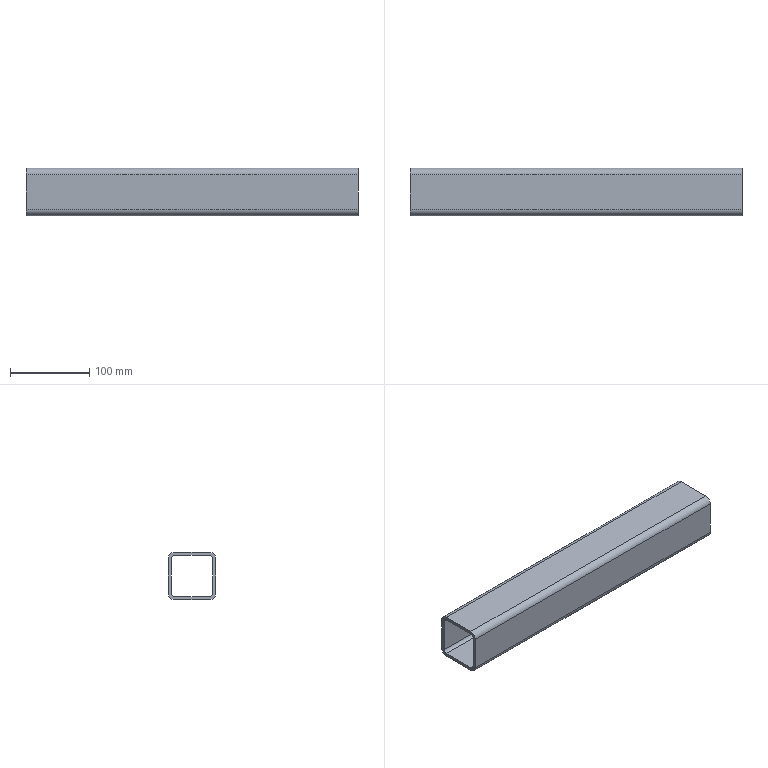Part | SolidWorks | features BaseBody 1 | 1 solid | 18 faces | box 420 x 60 x 60 mm | volume 359015 mm3 | plane 10 | cylinder 8 | commonest cylinder face diameters 8 x4 16 x4
STEP:
#1=CARTESIAN_POINT('',(-210.,2006.,-1308.));
#2=VERTEX_POINT('',#1);
#3=CARTESIAN_POINT('',(210.,2006.,-1308.));
#4=VERTEX_POINT('',#3);
#5=CARTESIAN_POINT('',(-240.,2006.,-1308.));
#6=DIRECTION('',(1.,0.,0.));
#7=VECTOR('',#6,1000.);
#8=LINE('',#5,#7);
#9=EDGE_CURVE('',#2,#4,#8,.T.);
#10=ORIENTED_EDGE('',*,*,#9,.T.);
#11=CARTESIAN_POINT('',(210.,2006.,-1352.));
#12=VERTEX_POINT('',#11);
#13=CARTESIAN_POINT('',(210.,2006.,-1308.));
#14=DIRECTION('',(0.,0.,-1.));
#15=VECTOR('',#14,1000.);
#16=LINE('',#13,#15);
#17=EDGE_CURVE('',#4,#12,#16,.T.);
#18=ORIENTED_EDGE('',*,*,#17,.T.);
#19=CARTESIAN_POINT('',(-210.,2006.,-1352.));
#20=VERTEX_POINT('',#19);
#21=CARTESIAN_POINT('',(-240.,2006.,-1352.));
#22=DIRECTION('',(-1.,0.,0.));
#23=VECTOR('',#22,1000.);
#24=LINE('',#21,#23);
#25=EDGE_CURVE('',#12,#20,#24,.T.);
#26=ORIENTED_EDGE('',*,*,#25,.T.);
#27=CARTESIAN_POINT('',(-210.,2006.,-1308.));
#28=DIRECTION('',(0.,0.,1.));
#29=VECTOR('',#28,1000.);
#30=LINE('',#27,#29);
#31=EDGE_CURVE('',#20,#2,#30,.T.);
#32=ORIENTED_EDGE('',*,*,#31,.T.);
#33=EDGE_LOOP('',(#10,#18,#26,#32));
#34=FACE_OUTER_BOUND('',#33,.T.);
#35=CARTESIAN_POINT('',(-240.,2006.,-1308.));
#36=DIRECTION('',(0.,1.,0.));
#37=DIRECTION('',(0.,0.,1.));
#38=AXIS2_PLACEMENT_3D('',#35,#36,#37);
#39=PLANE('',#38);
#40=ADVANCED_FACE('',(#34),#39,.T.);
#41=CARTESIAN_POINT('',(210.,2010.,-1304.));
#42=VERTEX_POINT('',#41);
#43=CARTESIAN_POINT('',(210.,2010.,-1308.));
#44=DIRECTION('',(1.,0.,0.));
#45=DIRECTION('',(0.,0.,-1.));
#46=AXIS2_PLACEMENT_3D('',#43,#44,#45);
#47=CIRCLE('',#46,4.);
#48=EDGE_CURVE('',#42,#4,#47,.T.);
#49=ORIENTED_EDGE('',*,*,#48,.F.);
#50=CARTESIAN_POINT('',(210.,2054.,-1304.));
#51=VERTEX_POINT('',#50);
#52=CARTESIAN_POINT('',(210.,2054.,-1304.));
#53=DIRECTION('',(0.,-1.,0.));
#54=VECTOR('',#53,1000.);
#55=LINE('',#52,#54);
#56=EDGE_CURVE('',#51,#42,#55,.T.);
#57=ORIENTED_EDGE('',*,*,#56,.F.);
#58=CARTESIAN_POINT('',(210.,2058.,-1308.));
#59=VERTEX_POINT('',#58);
#60=CARTESIAN_POINT('',(210.,2054.,-1308.));
#61=DIRECTION('',(1.,0.,0.));
#62=DIRECTION('',(0.,0.,-1.));
#63=AXIS2_PLACEMENT_3D('',#60,#61,#62);
#64=CIRCLE('',#63,4.);
#65=EDGE_CURVE('',#59,#51,#64,.T.);
#66=ORIENTED_EDGE('',*,*,#65,.F.);
#67=CARTESIAN_POINT('',(210.,2058.,-1352.));
#68=VERTEX_POINT('',#67);
#69=CARTESIAN_POINT('',(210.,2058.,-1352.));
#70=DIRECTION('',(0.,0.,1.));
#71=VECTOR('',#70,1000.);
#72=LINE('',#69,#71);
#73=EDGE_CURVE('',#68,#59,#72,.T.);
#74=ORIENTED_EDGE('',*,*,#73,.F.);
#75=CARTESIAN_POINT('',(210.,2054.,-1356.));
#76=VERTEX_POINT('',#75);
#77=CARTESIAN_POINT('',(210.,2054.,-1352.));
#78=DIRECTION('',(1.,0.,0.));
#79=DIRECTION('',(0.,0.,-1.));
#80=AXIS2_PLACEMENT_3D('',#77,#78,#79);
#81=CIRCLE('',#80,4.);
#82=EDGE_CURVE('',#76,#68,#81,.T.);
#83=ORIENTED_EDGE('',*,*,#82,.F.);
#84=CARTESIAN_POINT('',(210.,2010.,-1356.));
#85=VERTEX_POINT('',#84);
#86=CARTESIAN_POINT('',(210.,2054.,-1356.));
#87=DIRECTION('',(0.,1.,0.));
#88=VECTOR('',#87,1000.);
#89=LINE('',#86,#88);
#90=EDGE_CURVE('',#85,#76,#89,.T.);
#91=ORIENTED_EDGE('',*,*,#90,.F.);
#92=CARTESIAN_POINT('',(210.,2010.,-1352.));
#93=DIRECTION('',(1.,0.,0.));
#94=DIRECTION('',(0.,0.,-1.));
#95=AXIS2_PLACEMENT_3D('',#92,#93,#94);
#96=CIRCLE('',#95,4.);
#97=EDGE_CURVE('',#12,#85,#96,.T.);
#98=ORIENTED_EDGE('',*,*,#97,.F.);
#99=ORIENTED_EDGE('',*,*,#17,.F.);
#100=EDGE_LOOP('',(#49,#57,#66,#74,#83,#91,#98,#99));
#101=FACE_BOUND('',#100,.T.);
#102=CARTESIAN_POINT('',(210.,2054.,-1300.));
#103=VERTEX_POINT('',#102);
#104=CARTESIAN_POINT('',(210.,2062.,-1308.));
#105=VERTEX_POINT('',#104);
#106=CARTESIAN_POINT('',(210.,2054.,-1308.));
#107=DIRECTION('',(-1.,0.,0.));
#108=DIRECTION('',(0.,0.,-1.));
#109=AXIS2_PLACEMENT_3D('',#106,#107,#108);
#110=CIRCLE('',#109,8.);
#111=EDGE_CURVE('',#103,#105,#110,.T.);
#112=ORIENTED_EDGE('',*,*,#111,.F.);
#113=CARTESIAN_POINT('',(210.,2010.,-1300.));
#114=VERTEX_POINT('',#113);
#115=CARTESIAN_POINT('',(210.,2054.,-1300.));
#116=DIRECTION('',(0.,1.,0.));
#117=VECTOR('',#116,1000.);
#118=LINE('',#115,#117);
#119=EDGE_CURVE('',#114,#103,#118,.T.);
#120=ORIENTED_EDGE('',*,*,#119,.F.);
#121=CARTESIAN_POINT('',(210.,2002.,-1308.));
#122=VERTEX_POINT('',#121);
#123=CARTESIAN_POINT('',(210.,2010.,-1308.));
#124=DIRECTION('',(-1.,0.,0.));
#125=DIRECTION('',(0.,0.,-1.));
#126=AXIS2_PLACEMENT_3D('',#123,#124,#125);
#127=CIRCLE('',#126,8.);
#128=EDGE_CURVE('',#122,#114,#127,.T.);
#129=ORIENTED_EDGE('',*,*,#128,.F.);
#130=CARTESIAN_POINT('',(210.,2002.,-1352.));
#131=VERTEX_POINT('',#130);
#132=CARTESIAN_POINT('',(210.,2002.,-1352.));
#133=DIRECTION('',(0.,0.,1.));
#134=VECTOR('',#133,1000.);
#135=LINE('',#132,#134);
#136=EDGE_CURVE('',#131,#122,#135,.T.);
#137=ORIENTED_EDGE('',*,*,#136,.F.);
#138=CARTESIAN_POINT('',(210.,2010.,-1360.));
#139=VERTEX_POINT('',#138);
#140=CARTESIAN_POINT('',(210.,2010.,-1352.));
#141=DIRECTION('',(-1.,0.,0.));
#142=DIRECTION('',(0.,0.,-1.));
#143=AXIS2_PLACEMENT_3D('',#140,#141,#142);
#144=CIRCLE('',#143,8.);
#145=EDGE_CURVE('',#139,#131,#144,.T.);
#146=ORIENTED_EDGE('',*,*,#145,.F.);
#147=CARTESIAN_POINT('',(210.,2054.,-1360.));
#148=VERTEX_POINT('',#147);
#149=CARTESIAN_POINT('',(210.,2054.,-1360.));
#150=DIRECTION('',(0.,-1.,0.));
#151=VECTOR('',#150,1000.);
#152=LINE('',#149,#151);
#153=EDGE_CURVE('',#148,#139,#152,.T.);
#154=ORIENTED_EDGE('',*,*,#153,.F.);
#155=CARTESIAN_POINT('',(210.,2062.,-1352.));
#156=VERTEX_POINT('',#155);
#157=CARTESIAN_POINT('',(210.,2054.,-1352.));
#158=DIRECTION('',(-1.,0.,0.));
#159=DIRECTION('',(0.,0.,-1.));
#160=AXIS2_PLACEMENT_3D('',#157,#158,#159);
#161=CIRCLE('',#160,8.);
#162=EDGE_CURVE('',#156,#148,#161,.T.);
#163=ORIENTED_EDGE('',*,*,#162,.F.);
#164=CARTESIAN_POINT('',(210.,2062.,-1352.));
#165=DIRECTION('',(0.,0.,-1.));
#166=VECTOR('',#165,1000.);
#167=LINE('',#164,#166);
#168=EDGE_CURVE('',#105,#156,#167,.T.);
#169=ORIENTED_EDGE('',*,*,#168,.F.);
#170=EDGE_LOOP('',(#112,#120,#129,#137,#146,#154,#163,#169));
#171=FACE_OUTER_BOUND('',#170,.T.);
#172=CARTESIAN_POINT('',(210.,2054.,-1352.));
#173=DIRECTION('',(-1.,0.,0.));
#174=DIRECTION('',(0.,0.,1.));
#175=AXIS2_PLACEMENT_3D('',#172,#173,#174);
#176=PLANE('',#175);
#177=ADVANCED_FACE('',(#101,#171),#176,.F.);
#178=CARTESIAN_POINT('',(-210.,2010.,-1304.));
#179=VERTEX_POINT('',#178);
#180=CARTESIAN_POINT('',(-210.,2010.,-1308.));
#181=DIRECTION('',(1.,0.,0.));
#182=DIRECTION('',(0.,0.,-1.));
#183=AXIS2_PLACEMENT_3D('',#180,#181,#182);
#184=CIRCLE('',#183,4.);
#185=EDGE_CURVE('',#179,#2,#184,.T.);
#186=ORIENTED_EDGE('',*,*,#185,.F.);
#187=CARTESIAN_POINT('',(-240.,2010.,-1304.));
#188=DIRECTION('',(-1.,0.,0.));
#189=VECTOR('',#188,1000.);
#190=LINE('',#187,#189);
#191=EDGE_CURVE('',#42,#179,#190,.T.);
#192=ORIENTED_EDGE('',*,*,#191,.F.);
#193=ORIENTED_EDGE('',*,*,#48,.T.);
#194=ORIENTED_EDGE('',*,*,#9,.F.);
#195=EDGE_LOOP('',(#186,#192,#193,#194));
#196=FACE_OUTER_BOUND('',#195,.T.);
#197=CARTESIAN_POINT('',(-240.,2010.,-1308.));
#198=DIRECTION('',(1.,0.,0.));
#199=DIRECTION('',(0.,0.,-1.));
#200=AXIS2_PLACEMENT_3D('',#197,#198,#199);
#201=CYLINDRICAL_SURFACE('',#200,4.);
#202=ADVANCED_FACE('',(#196),#201,.F.);
#203=CARTESIAN_POINT('',(-210.,2058.,-1352.));
#204=VERTEX_POINT('',#203);
#205=CARTESIAN_POINT('',(-210.,2054.,-1356.));
#206=VERTEX_POINT('',#205);
#207=CARTESIAN_POINT('',(-210.,2054.,-1352.));
#208=DIRECTION('',(-1.,0.,0.));
#209=DIRECTION('',(0.,0.,-1.));
#210=AXIS2_PLACEMENT_3D('',#207,#208,#209);
#211=CIRCLE('',#210,4.);
#212=EDGE_CURVE('',#204,#206,#211,.T.);
#213=ORIENTED_EDGE('',*,*,#212,.F.);
#214=CARTESIAN_POINT('',(-210.,2058.,-1308.));
#215=VERTEX_POINT('',#214);
#216=CARTESIAN_POINT('',(-210.,2058.,-1330.));
#217=DIRECTION('',(0.,0.,-1.));
#218=VECTOR('',#217,1000.);
#219=LINE('',#216,#218);
#220=EDGE_CURVE('',#215,#204,#219,.T.);
#221=ORIENTED_EDGE('',*,*,#220,.F.);
#222=CARTESIAN_POINT('',(-210.,2054.,-1304.));
#223=VERTEX_POINT('',#222);
#224=CARTESIAN_POINT('',(-210.,2054.,-1308.));
#225=DIRECTION('',(-1.,0.,0.));
#226=DIRECTION('',(0.,0.,-1.));
#227=AXIS2_PLACEMENT_3D('',#224,#225,#226);
#228=CIRCLE('',#227,4.);
#229=EDGE_CURVE('',#223,#215,#228,.T.);
#230=ORIENTED_EDGE('',*,*,#229,.F.);
#231=CARTESIAN_POINT('',(-210.,1252.,-1304.));
#232=DIRECTION('',(0.,1.,0.));
#233=VECTOR('',#232,1000.);
#234=LINE('',#231,#233);
#235=EDGE_CURVE('',#179,#223,#234,.T.);
#236=ORIENTED_EDGE('',*,*,#235,.F.);
#237=ORIENTED_EDGE('',*,*,#185,.T.);
#238=ORIENTED_EDGE('',*,*,#31,.F.);
#239=CARTESIAN_POINT('',(-210.,2010.,-1356.));
#240=VERTEX_POINT('',#239);
#241=CARTESIAN_POINT('',(-210.,2010.,-1352.));
#242=DIRECTION('',(-1.,0.,0.));
#243=DIRECTION('',(0.,0.,-1.));
#244=AXIS2_PLACEMENT_3D('',#241,#242,#243);
#245=CIRCLE('',#244,4.);
#246=EDGE_CURVE('',#240,#20,#245,.T.);
#247=ORIENTED_EDGE('',*,*,#246,.F.);
#248=CARTESIAN_POINT('',(-210.,1252.,-1356.));
#249=DIRECTION('',(0.,-1.,0.));
#250=VECTOR('',#249,1000.);
#251=LINE('',#248,#250);
#252=EDGE_CURVE('',#206,#240,#251,.T.);
#253=ORIENTED_EDGE('',*,*,#252,.F.);
#254=EDGE_LOOP('',(#213,#221,#230,#236,#237,#238,#247,#253));
#255=FACE_BOUND('',#254,.T.);
#256=CARTESIAN_POINT('',(-210.,2002.,-1308.));
#257=VERTEX_POINT('',#256);
#258=CARTESIAN_POINT('',(-210.,2002.,-1352.));
#259=VERTEX_POINT('',#258);
#260=CARTESIAN_POINT('',(-210.,2002.,-1330.));
#261=DIRECTION('',(0.,0.,-1.));
#262=VECTOR('',#261,1000.);
#263=LINE('',#260,#262);
#264=EDGE_CURVE('',#257,#259,#263,.T.);
#265=ORIENTED_EDGE('',*,*,#264,.F.);
#266=CARTESIAN_POINT('',(-210.,2010.,-1300.));
#267=VERTEX_POINT('',#266);
#268=CARTESIAN_POINT('',(-210.,2010.,-1308.));
#269=DIRECTION('',(1.,0.,0.));
#270=DIRECTION('',(0.,0.,-1.));
#271=AXIS2_PLACEMENT_3D('',#268,#269,#270);
#272=CIRCLE('',#271,8.);
#273=EDGE_CURVE('',#267,#257,#272,.T.);
#274=ORIENTED_EDGE('',*,*,#273,.F.);
#275=CARTESIAN_POINT('',(-210.,2054.,-1300.));
#276=VERTEX_POINT('',#275);
#277=CARTESIAN_POINT('',(-210.,1252.,-1300.));
#278=DIRECTION('',(0.,-1.,0.));
#279=VECTOR('',#278,1000.);
#280=LINE('',#277,#279);
#281=EDGE_CURVE('',#276,#267,#280,.T.);
#282=ORIENTED_EDGE('',*,*,#281,.F.);
#283=CARTESIAN_POINT('',(-210.,2062.,-1308.));
#284=VERTEX_POINT('',#283);
#285=CARTESIAN_POINT('',(-210.,2054.,-1308.));
#286=DIRECTION('',(1.,0.,0.));
#287=DIRECTION('',(0.,0.,-1.));
#288=AXIS2_PLACEMENT_3D('',#285,#286,#287);
#289=CIRCLE('',#288,8.);
#290=EDGE_CURVE('',#284,#276,#289,.T.);
#291=ORIENTED_EDGE('',*,*,#290,.F.);
#292=CARTESIAN_POINT('',(-210.,2062.,-1352.));
#293=VERTEX_POINT('',#292);
#294=CARTESIAN_POINT('',(-210.,2062.,-1330.));
#295=DIRECTION('',(0.,0.,1.));
#296=VECTOR('',#295,1000.);
#297=LINE('',#294,#296);
#298=EDGE_CURVE('',#293,#284,#297,.T.);
#299=ORIENTED_EDGE('',*,*,#298,.F.);
#300=CARTESIAN_POINT('',(-210.,2054.,-1360.));
#301=VERTEX_POINT('',#300);
#302=CARTESIAN_POINT('',(-210.,2054.,-1352.));
#303=DIRECTION('',(1.,0.,0.));
#304=DIRECTION('',(0.,0.,-1.));
#305=AXIS2_PLACEMENT_3D('',#302,#303,#304);
#306=CIRCLE('',#305,8.);
#307=EDGE_CURVE('',#301,#293,#306,.T.);
#308=ORIENTED_EDGE('',*,*,#307,.F.);
#309=CARTESIAN_POINT('',(-210.,2010.,-1360.));
#310=VERTEX_POINT('',#309);
#311=CARTESIAN_POINT('',(-210.,1252.,-1360.));
#312=DIRECTION('',(0.,1.,0.));
#313=VECTOR('',#312,1000.);
#314=LINE('',#311,#313);
#315=EDGE_CURVE('',#310,#301,#314,.T.);
#316=ORIENTED_EDGE('',*,*,#315,.F.);
#317=CARTESIAN_POINT('',(-210.,2010.,-1352.));
#318=DIRECTION('',(1.,0.,0.));
#319=DIRECTION('',(0.,0.,-1.));
#320=AXIS2_PLACEMENT_3D('',#317,#318,#319);
#321=CIRCLE('',#320,8.);
#322=EDGE_CURVE('',#259,#310,#321,.T.);
#323=ORIENTED_EDGE('',*,*,#322,.F.);
#324=EDGE_LOOP('',(#265,#274,#282,#291,#299,#308,#316,#323));
#325=FACE_OUTER_BOUND('',#324,.T.);
#326=CARTESIAN_POINT('',(-210.,1252.,-1330.));
#327=DIRECTION('',(1.,0.,0.));
#328=DIRECTION('',(0.,0.,-1.));
#329=AXIS2_PLACEMENT_3D('',#326,#327,#328);
#330=PLANE('',#329);
#331=ADVANCED_FACE('',(#255,#325),#330,.F.);
#332=ORIENTED_EDGE('',*,*,#246,.T.);
#333=ORIENTED_EDGE('',*,*,#25,.F.);
#334=ORIENTED_EDGE('',*,*,#97,.T.);
#335=CARTESIAN_POINT('',(-240.,2010.,-1356.));
#336=DIRECTION('',(1.,0.,0.));
#337=VECTOR('',#336,1000.);
#338=LINE('',#335,#337);
#339=EDGE_CURVE('',#240,#85,#338,.T.);
#340=ORIENTED_EDGE('',*,*,#339,.F.);
#341=EDGE_LOOP('',(#332,#333,#334,#340));
#342=FACE_OUTER_BOUND('',#341,.T.);
#343=CARTESIAN_POINT('',(-240.,2010.,-1352.));
#344=DIRECTION('',(1.,0.,0.));
#345=DIRECTION('',(0.,0.,-1.));
#346=AXIS2_PLACEMENT_3D('',#343,#344,#345);
#347=CYLINDRICAL_SURFACE('',#346,4.);
#348=ADVANCED_FACE('',(#342),#347,.F.);
#349=CARTESIAN_POINT('',(-240.,2054.,-1304.));
#350=DIRECTION('',(1.,0.,0.));
#351=VECTOR('',#350,1000.);
#352=LINE('',#349,#351);
#353=EDGE_CURVE('',#223,#51,#352,.T.);
#354=ORIENTED_EDGE('',*,*,#353,.T.);
#355=ORIENTED_EDGE('',*,*,#56,.T.);
#356=ORIENTED_EDGE('',*,*,#191,.T.);
#357=ORIENTED_EDGE('',*,*,#235,.T.);
#358=EDGE_LOOP('',(#354,#355,#356,#357));
#359=FACE_OUTER_BOUND('',#358,.T.);
#360=CARTESIAN_POINT('',(-240.,2010.,-1304.));
#361=DIRECTION('',(0.,0.,-1.));
#362=DIRECTION('',(-1.,0.,0.));
#363=AXIS2_PLACEMENT_3D('',#360,#361,#362);
#364=PLANE('',#363);
#365=ADVANCED_FACE('',(#359),#364,.T.);
#366=ORIENTED_EDGE('',*,*,#229,.T.);
#367=CARTESIAN_POINT('',(-240.,2058.,-1308.));
#368=DIRECTION('',(-1.,0.,0.));
#369=VECTOR('',#368,1000.);
#370=LINE('',#367,#369);
#371=EDGE_CURVE('',#59,#215,#370,.T.);
#372=ORIENTED_EDGE('',*,*,#371,.F.);
#373=ORIENTED_EDGE('',*,*,#65,.T.);
#374=ORIENTED_EDGE('',*,*,#353,.F.);
#375=EDGE_LOOP('',(#366,#372,#373,#374));
#376=FACE_OUTER_BOUND('',#375,.T.);
#377=CARTESIAN_POINT('',(-240.,2054.,-1308.));
#378=DIRECTION('',(1.,0.,0.));
#379=DIRECTION('',(0.,0.,-1.));
#380=AXIS2_PLACEMENT_3D('',#377,#378,#379);
#381=CYLINDRICAL_SURFACE('',#380,4.);
#382=ADVANCED_FACE('',(#376),#381,.F.);
#383=CARTESIAN_POINT('',(-240.,2058.,-1352.));
#384=DIRECTION('',(1.,0.,0.));
#385=VECTOR('',#384,1000.);
#386=LINE('',#383,#385);
#387=EDGE_CURVE('',#204,#68,#386,.T.);
#388=ORIENTED_EDGE('',*,*,#387,.T.);
#389=ORIENTED_EDGE('',*,*,#73,.T.);
#390=ORIENTED_EDGE('',*,*,#371,.T.);
#391=ORIENTED_EDGE('',*,*,#220,.T.);
#392=EDGE_LOOP('',(#388,#389,#390,#391));
#393=FACE_OUTER_BOUND('',#392,.T.);
#394=CARTESIAN_POINT('',(-240.,2058.,-1352.));
#395=DIRECTION('',(0.,-1.,0.));
#396=DIRECTION('',(0.,0.,-1.));
#397=AXIS2_PLACEMENT_3D('',#394,#395,#396);
#398=PLANE('',#397);
#399=ADVANCED_FACE('',(#393),#398,.T.);
#400=ORIENTED_EDGE('',*,*,#212,.T.);
#401=CARTESIAN_POINT('',(-240.,2054.,-1356.));
#402=DIRECTION('',(-1.,0.,0.));
#403=VECTOR('',#402,1000.);
#404=LINE('',#401,#403);
#405=EDGE_CURVE('',#76,#206,#404,.T.);
#406=ORIENTED_EDGE('',*,*,#405,.F.);
#407=ORIENTED_EDGE('',*,*,#82,.T.);
#408=ORIENTED_EDGE('',*,*,#387,.F.);
#409=EDGE_LOOP('',(#400,#406,#407,#408));
#410=FACE_OUTER_BOUND('',#409,.T.);
#411=CARTESIAN_POINT('',(-240.,2054.,-1352.));
#412=DIRECTION('',(1.,0.,0.));
#413=DIRECTION('',(0.,0.,-1.));
#414=AXIS2_PLACEMENT_3D('',#411,#412,#413);
#415=CYLINDRICAL_SURFACE('',#414,4.);
#416=ADVANCED_FACE('',(#410),#415,.F.);
#417=ORIENTED_EDGE('',*,*,#339,.T.);
#418=ORIENTED_EDGE('',*,*,#90,.T.);
#419=ORIENTED_EDGE('',*,*,#405,.T.);
#420=ORIENTED_EDGE('',*,*,#252,.T.);
#421=EDGE_LOOP('',(#417,#418,#419,#420));
#422=FACE_OUTER_BOUND('',#421,.T.);
#423=CARTESIAN_POINT('',(-240.,2054.,-1356.));
#424=DIRECTION('',(0.,0.,1.));
#425=DIRECTION('',(1.,0.,0.));
#426=AXIS2_PLACEMENT_3D('',#423,#424,#425);
#427=PLANE('',#426);
#428=ADVANCED_FACE('',(#422),#427,.T.);
#429=CARTESIAN_POINT('',(-240.,2062.,-1352.));
#430=DIRECTION('',(1.,0.,0.));
#431=VECTOR('',#430,1000.);
#432=LINE('',#429,#431);
#433=EDGE_CURVE('',#293,#156,#432,.T.);
#434=ORIENTED_EDGE('',*,*,#433,.F.);
#435=ORIENTED_EDGE('',*,*,#298,.T.);
#436=CARTESIAN_POINT('',(-240.,2062.,-1308.));
#437=DIRECTION('',(-1.,0.,0.));
#438=VECTOR('',#437,1000.);
#439=LINE('',#436,#438);
#440=EDGE_CURVE('',#105,#284,#439,.T.);
#441=ORIENTED_EDGE('',*,*,#440,.F.);
#442=ORIENTED_EDGE('',*,*,#168,.T.);
#443=EDGE_LOOP('',(#434,#435,#441,#442));
#444=FACE_OUTER_BOUND('',#443,.T.);
#445=CARTESIAN_POINT('',(-240.,2062.,-1352.));
#446=DIRECTION('',(0.,-1.,0.));
#447=DIRECTION('',(0.,0.,-1.));
#448=AXIS2_PLACEMENT_3D('',#445,#446,#447);
#449=PLANE('',#448);
#450=ADVANCED_FACE('',(#444),#449,.F.);
#451=ORIENTED_EDGE('',*,*,#290,.T.);
#452=CARTESIAN_POINT('',(-240.,2054.,-1300.));
#453=DIRECTION('',(1.,0.,0.));
#454=VECTOR('',#453,1000.);
#455=LINE('',#452,#454);
#456=EDGE_CURVE('',#276,#103,#455,.T.);
#457=ORIENTED_EDGE('',*,*,#456,.T.);
#458=ORIENTED_EDGE('',*,*,#111,.T.);
#459=ORIENTED_EDGE('',*,*,#440,.T.);
#460=EDGE_LOOP('',(#451,#457,#458,#459));
#461=FACE_OUTER_BOUND('',#460,.T.);
#462=CARTESIAN_POINT('',(-240.,2054.,-1308.));
#463=DIRECTION('',(1.,0.,0.));
#464=DIRECTION('',(0.,0.,-1.));
#465=AXIS2_PLACEMENT_3D('',#462,#463,#464);
#466=CYLINDRICAL_SURFACE('',#465,8.);
#467=ADVANCED_FACE('',(#461),#466,.T.);
#468=ORIENTED_EDGE('',*,*,#456,.F.);
#469=ORIENTED_EDGE('',*,*,#281,.T.);
#470=CARTESIAN_POINT('',(-240.,2010.,-1300.));
#471=DIRECTION('',(-1.,0.,0.));
#472=VECTOR('',#471,1000.);
#473=LINE('',#470,#472);
#474=EDGE_CURVE('',#114,#267,#473,.T.);
#475=ORIENTED_EDGE('',*,*,#474,.F.);
#476=ORIENTED_EDGE('',*,*,#119,.T.);
#477=EDGE_LOOP('',(#468,#469,#475,#476));
#478=FACE_OUTER_BOUND('',#477,.T.);
#479=CARTESIAN_POINT('',(-240.,2010.,-1300.));
#480=DIRECTION('',(0.,0.,-1.));
#481=DIRECTION('',(-1.,0.,0.));
#482=AXIS2_PLACEMENT_3D('',#479,#480,#481);
#483=PLANE('',#482);
#484=ADVANCED_FACE('',(#478),#483,.F.);
#485=ORIENTED_EDGE('',*,*,#273,.T.);
#486=CARTESIAN_POINT('',(-240.,2002.,-1308.));
#487=DIRECTION('',(1.,0.,0.));
#488=VECTOR('',#487,1000.);
#489=LINE('',#486,#488);
#490=EDGE_CURVE('',#257,#122,#489,.T.);
#491=ORIENTED_EDGE('',*,*,#490,.T.);
#492=ORIENTED_EDGE('',*,*,#128,.T.);
#493=ORIENTED_EDGE('',*,*,#474,.T.);
#494=EDGE_LOOP('',(#485,#491,#492,#493));
#495=FACE_OUTER_BOUND('',#494,.T.);
#496=CARTESIAN_POINT('',(-240.,2010.,-1308.));
#497=DIRECTION('',(1.,0.,0.));
#498=DIRECTION('',(0.,0.,-1.));
#499=AXIS2_PLACEMENT_3D('',#496,#497,#498);
#500=CYLINDRICAL_SURFACE('',#499,8.);
#501=ADVANCED_FACE('',(#495),#500,.T.);
#502=ORIENTED_EDGE('',*,*,#490,.F.);
#503=ORIENTED_EDGE('',*,*,#264,.T.);
#504=CARTESIAN_POINT('',(-240.,2002.,-1352.));
#505=DIRECTION('',(-1.,0.,0.));
#506=VECTOR('',#505,1000.);
#507=LINE('',#504,#506);
#508=EDGE_CURVE('',#131,#259,#507,.T.);
#509=ORIENTED_EDGE('',*,*,#508,.F.);
#510=ORIENTED_EDGE('',*,*,#136,.T.);
#511=EDGE_LOOP('',(#502,#503,#509,#510));
#512=FACE_OUTER_BOUND('',#511,.T.);
#513=CARTESIAN_POINT('',(-240.,2002.,-1308.));
#514=DIRECTION('',(0.,1.,0.));
#515=DIRECTION('',(0.,0.,1.));
#516=AXIS2_PLACEMENT_3D('',#513,#514,#515);
#517=PLANE('',#516);
#518=ADVANCED_FACE('',(#512),#517,.F.);
#519=ORIENTED_EDGE('',*,*,#322,.T.);
#520=CARTESIAN_POINT('',(-240.,2010.,-1360.));
#521=DIRECTION('',(1.,0.,0.));
#522=VECTOR('',#521,1000.);
#523=LINE('',#520,#522);
#524=EDGE_CURVE('',#310,#139,#523,.T.);
#525=ORIENTED_EDGE('',*,*,#524,.T.);
#526=ORIENTED_EDGE('',*,*,#145,.T.);
#527=ORIENTED_EDGE('',*,*,#508,.T.);
#528=EDGE_LOOP('',(#519,#525,#526,#527));
#529=FACE_OUTER_BOUND('',#528,.T.);
#530=CARTESIAN_POINT('',(-240.,2010.,-1352.));
#531=DIRECTION('',(1.,0.,0.));
#532=DIRECTION('',(0.,0.,-1.));
#533=AXIS2_PLACEMENT_3D('',#530,#531,#532);
#534=CYLINDRICAL_SURFACE('',#533,8.);
#535=ADVANCED_FACE('',(#529),#534,.T.);
#536=ORIENTED_EDGE('',*,*,#524,.F.);
#537=ORIENTED_EDGE('',*,*,#315,.T.);
#538=CARTESIAN_POINT('',(-240.,2054.,-1360.));
#539=DIRECTION('',(-1.,0.,0.));
#540=VECTOR('',#539,1000.);
#541=LINE('',#538,#540);
#542=EDGE_CURVE('',#148,#301,#541,.T.);
#543=ORIENTED_EDGE('',*,*,#542,.F.);
#544=ORIENTED_EDGE('',*,*,#153,.T.);
#545=EDGE_LOOP('',(#536,#537,#543,#544));
#546=FACE_OUTER_BOUND('',#545,.T.);
#547=CARTESIAN_POINT('',(-240.,2054.,-1360.));
#548=DIRECTION('',(0.,0.,1.));
#549=DIRECTION('',(1.,0.,0.));
#550=AXIS2_PLACEMENT_3D('',#547,#548,#549);
#551=PLANE('',#550);
#552=ADVANCED_FACE('',(#546),#551,.F.);
#553=ORIENTED_EDGE('',*,*,#307,.T.);
#554=ORIENTED_EDGE('',*,*,#433,.T.);
#555=ORIENTED_EDGE('',*,*,#162,.T.);
#556=ORIENTED_EDGE('',*,*,#542,.T.);
#557=EDGE_LOOP('',(#553,#554,#555,#556));
#558=FACE_OUTER_BOUND('',#557,.T.);
#559=CARTESIAN_POINT('',(-240.,2054.,-1352.));
#560=DIRECTION('',(1.,0.,0.));
#561=DIRECTION('',(0.,0.,-1.));
#562=AXIS2_PLACEMENT_3D('',#559,#560,#561);
#563=CYLINDRICAL_SURFACE('',#562,8.);
#564=ADVANCED_FACE('',(#558),#563,.T.);
#565=CLOSED_SHELL('',(#40,#177,#202,#331,#348,#365,#382,#399,#416,#428,#450,#467,#484,#501,#518,#535,#552,#564));
#566=MANIFOLD_SOLID_BREP('',#565);
#567=CARTESIAN_POINT('',(0.,0.,0.));
#568=DIRECTION('',(0.,0.,1.));
#569=DIRECTION('',(1.,0.,0.));
#570=AXIS2_PLACEMENT_3D('',#567,#568,#569);
#571=(LENGTH_UNIT()NAMED_UNIT(*)SI_UNIT(.MILLI.,.METRE.));
#572=UNCERTAINTY_MEASURE_WITH_UNIT(LENGTH_MEASURE(0.00001),#571,'','');
#573=(NAMED_UNIT(*)PLANE_ANGLE_UNIT()SI_UNIT($,.RADIAN.));
#574=(NAMED_UNIT(*)SI_UNIT($,.STERADIAN.)SOLID_ANGLE_UNIT());
#575=(GEOMETRIC_REPRESENTATION_CONTEXT(3)GLOBAL_UNCERTAINTY_ASSIGNED_CONTEXT((#572))GLOBAL_UNIT_ASSIGNED_CONTEXT((#571,#573,#574))REPRESENTATION_CONTEXT('',''));
#576=ADVANCED_BREP_SHAPE_REPRESENTATION('',(#566,#570),#575);